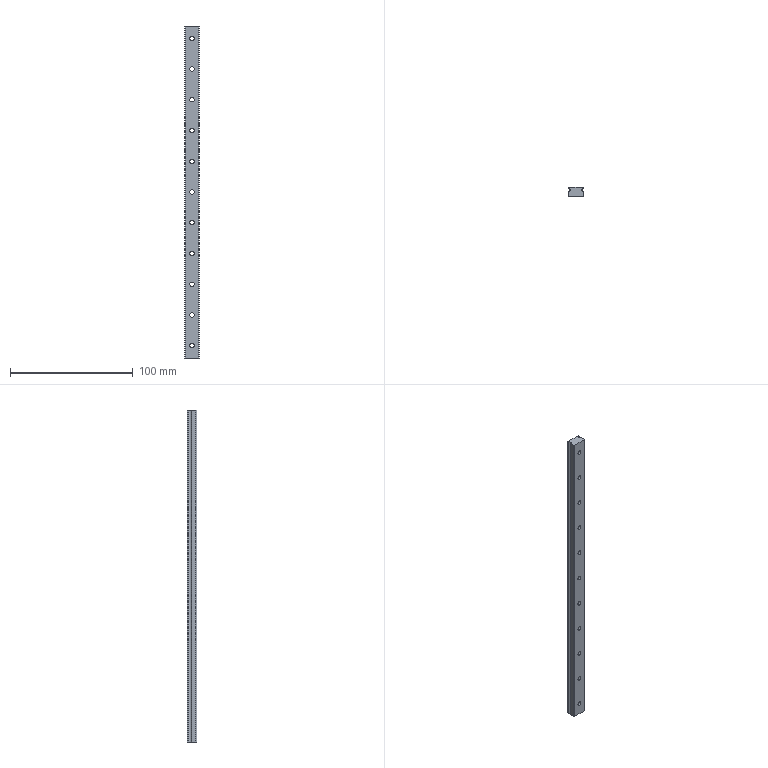Part | STEP file | QA-r_SE2BL13_270 | 1 solid | 68 faces | box 12 x 7.5 x 270 mm | volume 21190 mm3 | cylinder 47 | plane 21 | commonest cylinder face diameters 3.5 x22 6 x22 2.5 x3